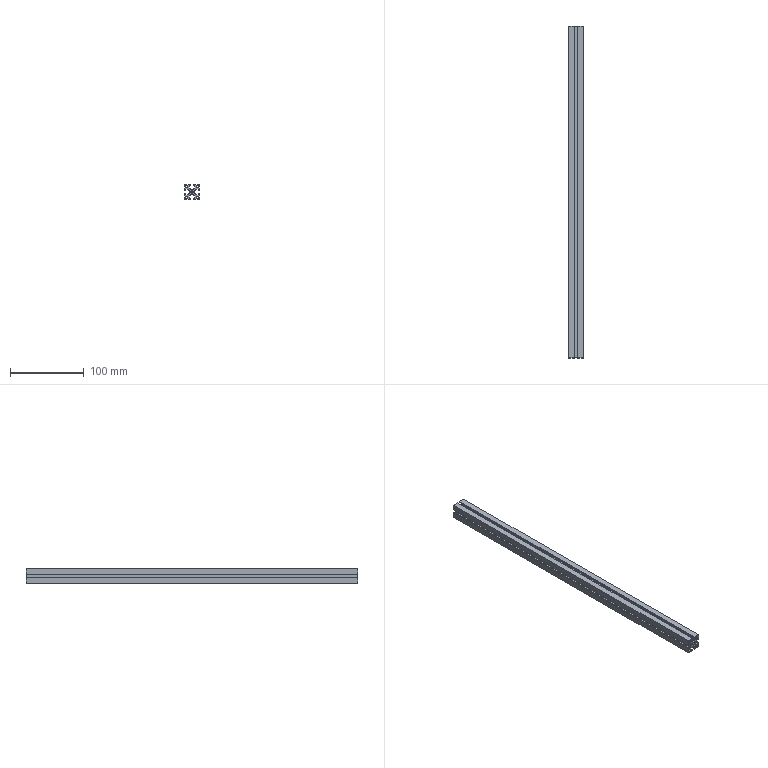Part | STEP file | 20 aluminium profile transverse 2 | 1 solid | 64 faces | box 20 x 450 x 20 mm | volume 80001 mm3 | plane 54 | cylinder 10 | commonest cylinder face diameters 3.3 x10